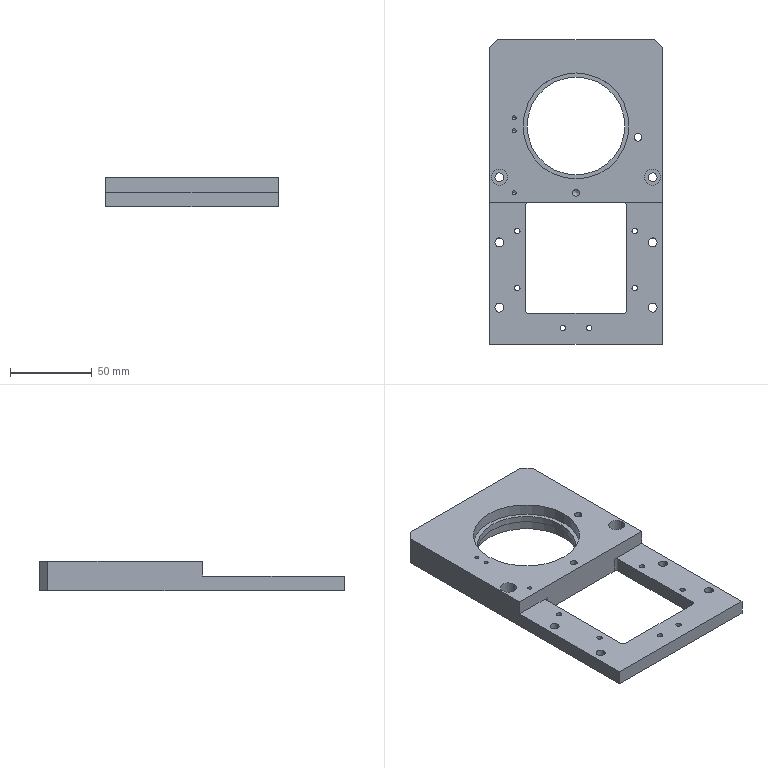Part | SolidWorks | features HoleWzd 7, ICE 4, Chamfer 1, Cut 1, Extrusion 1, Fillet 1 | 1 solid | 84 faces | box 106 x 187 x 18 mm | volume 173548 mm3 | cylinder 54 | plane 18 | cone 12 | commonest cylinder face diameters 3.3 x16 5.5 x12 2.5 x6 4 x4 10 x4 65 x4